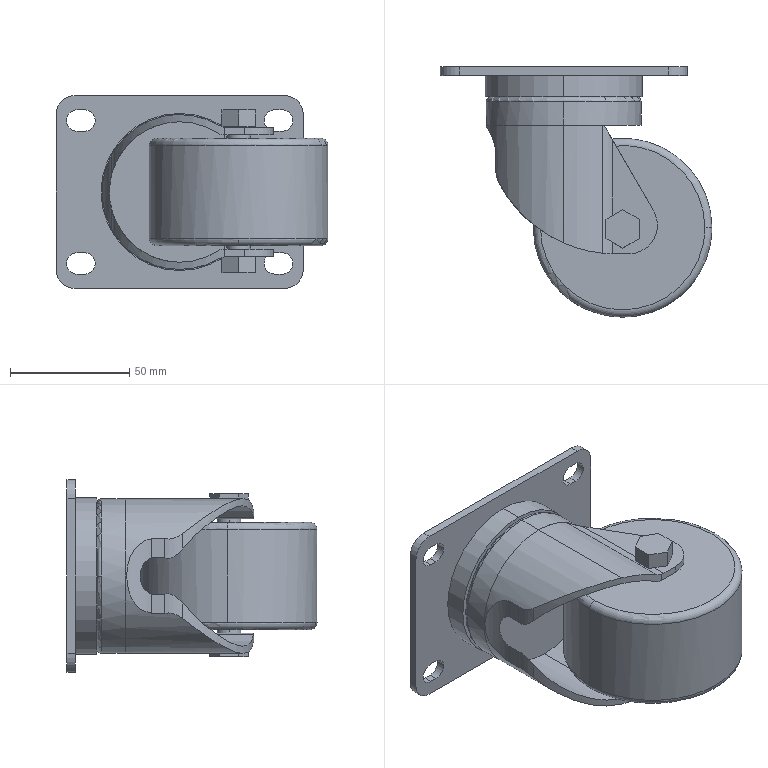Part | STEP file | SK6-U75105BP-3 inch heavy-duty caster | 1 solid | 100 faces | box 114.176 x 105 x 81 mm | volume 325491 mm3 | cylinder 47 | plane 47 | torus 6 | commonest cylinder face diameters 9 x10 16 x8 10 x6 24 x4 59 x3 65 x3